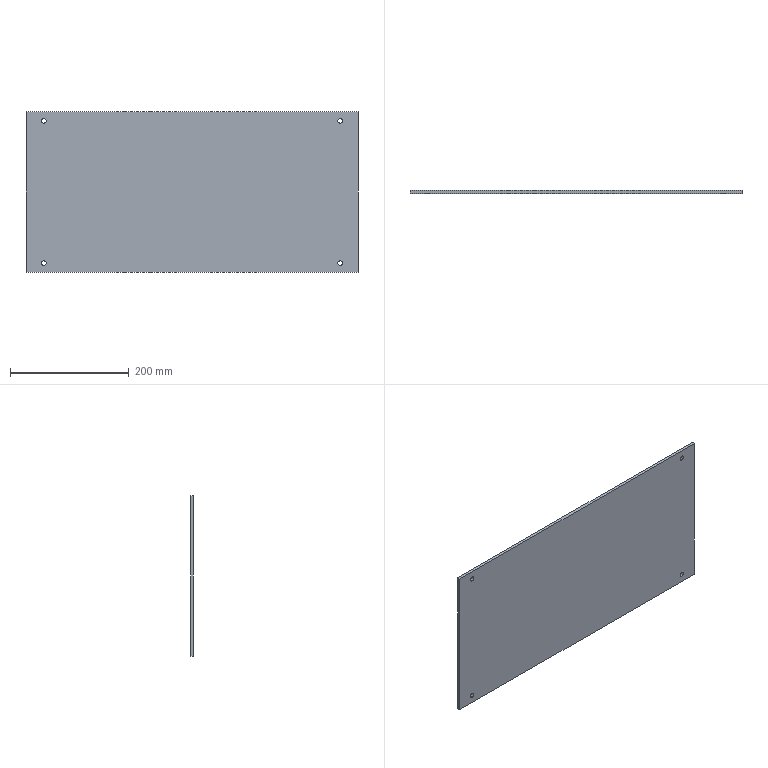Part | STEP file | OP10-004_front cover (L) | 1 solid | 14 faces | box 560 x 5 x 270 mm | volume 754995 mm3 | cylinder 8 | plane 6 | commonest cylinder face diameters 8 x8
STEP:
#1=CARTESIAN_POINT('',(0.,0.,0.));
#2=DIRECTION('',(0.,0.,1.));
#3=DIRECTION('',(1.,0.,0.));
#4=AXIS2_PLACEMENT_3D('',#1,#2,#3);
#5=CARTESIAN_POINT('',(250.,0.,124.));
#6=VERTEX_POINT('',#5);
#7=CARTESIAN_POINT('',(250.,5.,124.));
#8=VERTEX_POINT('',#7);
#9=CARTESIAN_POINT('',(250.,5.,124.));
#10=DIRECTION('',(0.,1.,0.));
#11=VECTOR('',#10,1.);
#12=LINE('',#9,#11);
#13=CARTESIAN_POINT('',(250.,5.,120.));
#14=DIRECTION('',(0.,1.,0.));
#15=DIRECTION('',(0.,0.,1.));
#16=AXIS2_PLACEMENT_3D('',#13,#14,#15);
#17=CYLINDRICAL_SURFACE('',#16,4.);
#18=CARTESIAN_POINT('',(6.283,0.));
#19=DIRECTION('',(0.,1.));
#20=VECTOR('',#19,1.);
#21=LINE('',#18,#20);
#22=(GEOMETRIC_REPRESENTATION_CONTEXT(2)PARAMETRIC_REPRESENTATION_CONTEXT()REPRESENTATION_CONTEXT('',''));
#23=DEFINITIONAL_REPRESENTATION('',(#21),#22);
#24=PCURVE('',#17,#23);
#25=CARTESIAN_POINT('',(250.,5.,120.));
#26=DIRECTION('',(0.,1.,0.));
#27=DIRECTION('',(0.,0.,1.));
#28=AXIS2_PLACEMENT_3D('',#25,#26,#27);
#29=CYLINDRICAL_SURFACE('',#28,4.);
#30=CARTESIAN_POINT('',(0.,0.));
#31=DIRECTION('',(0.,1.));
#32=VECTOR('',#31,1.);
#33=LINE('',#30,#32);
#34=(GEOMETRIC_REPRESENTATION_CONTEXT(2)PARAMETRIC_REPRESENTATION_CONTEXT()REPRESENTATION_CONTEXT('',''));
#35=DEFINITIONAL_REPRESENTATION('',(#33),#34);
#36=PCURVE('',#29,#35);
#37=SURFACE_CURVE('',#12,(#24,#36),.PCURVE_S1.);
#38=EDGE_CURVE('',#6,#8,#37,.T.);
#39=ORIENTED_EDGE('',*,*,#38,.T.);
#40=CARTESIAN_POINT('',(250.,5.,116.));
#41=VERTEX_POINT('',#40);
#42=CARTESIAN_POINT('',(250.,5.,120.));
#43=DIRECTION('',(0.,1.,0.));
#44=DIRECTION('',(0.,0.,1.));
#45=AXIS2_PLACEMENT_3D('',#42,#43,#44);
#46=CIRCLE('',#45,4.);
#47=CARTESIAN_POINT('',(0.,0.));
#48=DIRECTION('',(1.,0.));
#49=VECTOR('',#48,1.);
#50=LINE('',#47,#49);
#51=(GEOMETRIC_REPRESENTATION_CONTEXT(2)PARAMETRIC_REPRESENTATION_CONTEXT()REPRESENTATION_CONTEXT('',''));
#52=DEFINITIONAL_REPRESENTATION('',(#50),#51);
#53=PCURVE('',#17,#52);
#54=CARTESIAN_POINT('',(0.,5.,0.));
#55=DIRECTION('',(0.,-1.,0.));
#56=DIRECTION('',(0.,0.,-1.));
#57=AXIS2_PLACEMENT_3D('',#54,#55,#56);
#58=PLANE('',#57);
#59=CARTESIAN_POINT('',(-124.,250.));
#60=CARTESIAN_POINT('',(-124.,256.928));
#61=CARTESIAN_POINT('',(-118.,253.464));
#62=CARTESIAN_POINT('',(-112.,250.));
#63=CARTESIAN_POINT('',(-118.,246.536));
#64=CARTESIAN_POINT('',(-124.,243.072));
#65=CARTESIAN_POINT('',(-124.,250.));
#66=(BOUNDED_CURVE()B_SPLINE_CURVE(2,(#59,#60,#61,#62,#63,#64,#65),.UNSPECIFIED.,.T.,.F.)B_SPLINE_CURVE_WITH_KNOTS((1,2,2,2,2,1),(-2.094,0.,2.094,4.189,6.283,8.378),.UNSPECIFIED.)CURVE()GEOMETRIC_REPRESENTATION_ITEM()RATIONAL_B_SPLINE_CURVE((1.,0.5,1.,0.5,1.,0.5,1.))REPRESENTATION_ITEM(''));
#67=(GEOMETRIC_REPRESENTATION_CONTEXT(2)PARAMETRIC_REPRESENTATION_CONTEXT()REPRESENTATION_CONTEXT('',''));
#68=DEFINITIONAL_REPRESENTATION('',(#66),#67);
#69=PCURVE('',#58,#68);
#70=SURFACE_CURVE('',#46,(#53,#69),.PCURVE_S1.);
#71=EDGE_CURVE('',#41,#8,#70,.T.);
#72=ORIENTED_EDGE('',*,*,#71,.F.);
#73=CARTESIAN_POINT('',(250.,0.,116.));
#74=VERTEX_POINT('',#73);
#75=CARTESIAN_POINT('',(250.,5.,116.));
#76=DIRECTION('',(0.,1.,0.));
#77=VECTOR('',#76,1.);
#78=LINE('',#75,#77);
#79=CARTESIAN_POINT('',(3.142,0.));
#80=DIRECTION('',(0.,1.));
#81=VECTOR('',#80,1.);
#82=LINE('',#79,#81);
#83=(GEOMETRIC_REPRESENTATION_CONTEXT(2)PARAMETRIC_REPRESENTATION_CONTEXT()REPRESENTATION_CONTEXT('',''));
#84=DEFINITIONAL_REPRESENTATION('',(#82),#83);
#85=PCURVE('',#17,#84);
#86=CARTESIAN_POINT('',(3.142,0.));
#87=DIRECTION('',(0.,1.));
#88=VECTOR('',#87,1.);
#89=LINE('',#86,#88);
#90=(GEOMETRIC_REPRESENTATION_CONTEXT(2)PARAMETRIC_REPRESENTATION_CONTEXT()REPRESENTATION_CONTEXT('',''));
#91=DEFINITIONAL_REPRESENTATION('',(#89),#90);
#92=PCURVE('',#29,#91);
#93=SURFACE_CURVE('',#78,(#85,#92),.PCURVE_S1.);
#94=EDGE_CURVE('',#74,#41,#93,.T.);
#95=ORIENTED_EDGE('',*,*,#94,.F.);
#96=CARTESIAN_POINT('',(250.,0.,120.));
#97=DIRECTION('',(0.,-1.,0.));
#98=DIRECTION('',(0.,0.,-1.));
#99=AXIS2_PLACEMENT_3D('',#96,#97,#98);
#100=CIRCLE('',#99,4.);
#101=CARTESIAN_POINT('',(9.425,-5.));
#102=DIRECTION('',(-1.,0.));
#103=VECTOR('',#102,1.);
#104=LINE('',#101,#103);
#105=(GEOMETRIC_REPRESENTATION_CONTEXT(2)PARAMETRIC_REPRESENTATION_CONTEXT()REPRESENTATION_CONTEXT('',''));
#106=DEFINITIONAL_REPRESENTATION('',(#104),#105);
#107=PCURVE('',#17,#106);
#108=CARTESIAN_POINT('',(0.,0.,0.));
#109=DIRECTION('',(0.,-1.,0.));
#110=DIRECTION('',(0.,0.,-1.));
#111=AXIS2_PLACEMENT_3D('',#108,#109,#110);
#112=PLANE('',#111);
#113=CARTESIAN_POINT('',(-120.,250.));
#114=DIRECTION('',(1.,0.));
#115=AXIS2_PLACEMENT_2D('',#113,#114);
#116=CIRCLE('',#115,4.);
#117=(GEOMETRIC_REPRESENTATION_CONTEXT(2)PARAMETRIC_REPRESENTATION_CONTEXT()REPRESENTATION_CONTEXT('',''));
#118=DEFINITIONAL_REPRESENTATION('',(#116),#117);
#119=PCURVE('',#112,#118);
#120=SURFACE_CURVE('',#100,(#107,#119),.PCURVE_S1.);
#121=EDGE_CURVE('',#6,#74,#120,.T.);
#122=ORIENTED_EDGE('',*,*,#121,.F.);
#123=EDGE_LOOP('',(#39,#72,#95,#122));
#124=FACE_BOUND('',#123,.F.);
#125=ADVANCED_FACE('',(#124),#17,.F.);
#126=CARTESIAN_POINT('',(-250.,0.,124.));
#127=VERTEX_POINT('',#126);
#128=CARTESIAN_POINT('',(-250.,5.,124.));
#129=VERTEX_POINT('',#128);
#130=CARTESIAN_POINT('',(-250.,5.,124.));
#131=DIRECTION('',(0.,1.,0.));
#132=VECTOR('',#131,1.);
#133=LINE('',#130,#132);
#134=CARTESIAN_POINT('',(-250.,5.,120.));
#135=DIRECTION('',(0.,1.,0.));
#136=DIRECTION('',(0.,0.,1.));
#137=AXIS2_PLACEMENT_3D('',#134,#135,#136);
#138=CYLINDRICAL_SURFACE('',#137,4.);
#139=CARTESIAN_POINT('',(6.283,0.));
#140=DIRECTION('',(0.,1.));
#141=VECTOR('',#140,1.);
#142=LINE('',#139,#141);
#143=(GEOMETRIC_REPRESENTATION_CONTEXT(2)PARAMETRIC_REPRESENTATION_CONTEXT()REPRESENTATION_CONTEXT('',''));
#144=DEFINITIONAL_REPRESENTATION('',(#142),#143);
#145=PCURVE('',#138,#144);
#146=CARTESIAN_POINT('',(-250.,5.,120.));
#147=DIRECTION('',(0.,1.,0.));
#148=DIRECTION('',(0.,0.,1.));
#149=AXIS2_PLACEMENT_3D('',#146,#147,#148);
#150=CYLINDRICAL_SURFACE('',#149,4.);
#151=CARTESIAN_POINT('',(0.,0.));
#152=DIRECTION('',(0.,1.));
#153=VECTOR('',#152,1.);
#154=LINE('',#151,#153);
#155=(GEOMETRIC_REPRESENTATION_CONTEXT(2)PARAMETRIC_REPRESENTATION_CONTEXT()REPRESENTATION_CONTEXT('',''));
#156=DEFINITIONAL_REPRESENTATION('',(#154),#155);
#157=PCURVE('',#150,#156);
#158=SURFACE_CURVE('',#133,(#145,#157),.PCURVE_S1.);
#159=EDGE_CURVE('',#127,#129,#158,.T.);
#160=ORIENTED_EDGE('',*,*,#159,.T.);
#161=CARTESIAN_POINT('',(-250.,5.,116.));
#162=VERTEX_POINT('',#161);
#163=CARTESIAN_POINT('',(-250.,5.,120.));
#164=DIRECTION('',(0.,1.,0.));
#165=DIRECTION('',(0.,0.,1.));
#166=AXIS2_PLACEMENT_3D('',#163,#164,#165);
#167=CIRCLE('',#166,4.);
#168=CARTESIAN_POINT('',(0.,0.));
#169=DIRECTION('',(1.,0.));
#170=VECTOR('',#169,1.);
#171=LINE('',#168,#170);
#172=(GEOMETRIC_REPRESENTATION_CONTEXT(2)PARAMETRIC_REPRESENTATION_CONTEXT()REPRESENTATION_CONTEXT('',''));
#173=DEFINITIONAL_REPRESENTATION('',(#171),#172);
#174=PCURVE('',#138,#173);
#175=CARTESIAN_POINT('',(-124.,-250.));
#176=CARTESIAN_POINT('',(-124.,-243.072));
#177=CARTESIAN_POINT('',(-118.,-246.536));
#178=CARTESIAN_POINT('',(-112.,-250.));
#179=CARTESIAN_POINT('',(-118.,-253.464));
#180=CARTESIAN_POINT('',(-124.,-256.928));
#181=CARTESIAN_POINT('',(-124.,-250.));
#182=(BOUNDED_CURVE()B_SPLINE_CURVE(2,(#175,#176,#177,#178,#179,#180,#181),.UNSPECIFIED.,.T.,.F.)B_SPLINE_CURVE_WITH_KNOTS((1,2,2,2,2,1),(-2.094,0.,2.094,4.189,6.283,8.378),.UNSPECIFIED.)CURVE()GEOMETRIC_REPRESENTATION_ITEM()RATIONAL_B_SPLINE_CURVE((1.,0.5,1.,0.5,1.,0.5,1.))REPRESENTATION_ITEM(''));
#183=(GEOMETRIC_REPRESENTATION_CONTEXT(2)PARAMETRIC_REPRESENTATION_CONTEXT()REPRESENTATION_CONTEXT('',''));
#184=DEFINITIONAL_REPRESENTATION('',(#182),#183);
#185=PCURVE('',#58,#184);
#186=SURFACE_CURVE('',#167,(#174,#185),.PCURVE_S1.);
#187=EDGE_CURVE('',#162,#129,#186,.T.);
#188=ORIENTED_EDGE('',*,*,#187,.F.);
#189=CARTESIAN_POINT('',(-250.,0.,116.));
#190=VERTEX_POINT('',#189);
#191=CARTESIAN_POINT('',(-250.,5.,116.));
#192=DIRECTION('',(0.,1.,0.));
#193=VECTOR('',#192,1.);
#194=LINE('',#191,#193);
#195=CARTESIAN_POINT('',(3.142,0.));
#196=DIRECTION('',(0.,1.));
#197=VECTOR('',#196,1.);
#198=LINE('',#195,#197);
#199=(GEOMETRIC_REPRESENTATION_CONTEXT(2)PARAMETRIC_REPRESENTATION_CONTEXT()REPRESENTATION_CONTEXT('',''));
#200=DEFINITIONAL_REPRESENTATION('',(#198),#199);
#201=PCURVE('',#138,#200);
#202=CARTESIAN_POINT('',(3.142,0.));
#203=DIRECTION('',(0.,1.));
#204=VECTOR('',#203,1.);
#205=LINE('',#202,#204);
#206=(GEOMETRIC_REPRESENTATION_CONTEXT(2)PARAMETRIC_REPRESENTATION_CONTEXT()REPRESENTATION_CONTEXT('',''));
#207=DEFINITIONAL_REPRESENTATION('',(#205),#206);
#208=PCURVE('',#150,#207);
#209=SURFACE_CURVE('',#194,(#201,#208),.PCURVE_S1.);
#210=EDGE_CURVE('',#190,#162,#209,.T.);
#211=ORIENTED_EDGE('',*,*,#210,.F.);
#212=CARTESIAN_POINT('',(-250.,0.,120.));
#213=DIRECTION('',(0.,-1.,0.));
#214=DIRECTION('',(0.,0.,-1.));
#215=AXIS2_PLACEMENT_3D('',#212,#213,#214);
#216=CIRCLE('',#215,4.);
#217=CARTESIAN_POINT('',(9.425,-5.));
#218=DIRECTION('',(-1.,0.));
#219=VECTOR('',#218,1.);
#220=LINE('',#217,#219);
#221=(GEOMETRIC_REPRESENTATION_CONTEXT(2)PARAMETRIC_REPRESENTATION_CONTEXT()REPRESENTATION_CONTEXT('',''));
#222=DEFINITIONAL_REPRESENTATION('',(#220),#221);
#223=PCURVE('',#138,#222);
#224=CARTESIAN_POINT('',(-120.,-250.));
#225=DIRECTION('',(1.,0.));
#226=AXIS2_PLACEMENT_2D('',#224,#225);
#227=CIRCLE('',#226,4.);
#228=(GEOMETRIC_REPRESENTATION_CONTEXT(2)PARAMETRIC_REPRESENTATION_CONTEXT()REPRESENTATION_CONTEXT('',''));
#229=DEFINITIONAL_REPRESENTATION('',(#227),#228);
#230=PCURVE('',#112,#229);
#231=SURFACE_CURVE('',#216,(#223,#230),.PCURVE_S1.);
#232=EDGE_CURVE('',#127,#190,#231,.T.);
#233=ORIENTED_EDGE('',*,*,#232,.F.);
#234=EDGE_LOOP('',(#160,#188,#211,#233));
#235=FACE_BOUND('',#234,.F.);
#236=ADVANCED_FACE('',(#235),#138,.F.);
#237=CARTESIAN_POINT('',(250.,0.,-116.));
#238=VERTEX_POINT('',#237);
#239=CARTESIAN_POINT('',(250.,5.,-116.));
#240=VERTEX_POINT('',#239);
#241=CARTESIAN_POINT('',(250.,5.,-116.));
#242=DIRECTION('',(0.,1.,0.));
#243=VECTOR('',#242,1.);
#244=LINE('',#241,#243);
#245=CARTESIAN_POINT('',(250.,5.,-120.));
#246=DIRECTION('',(0.,1.,0.));
#247=DIRECTION('',(0.,0.,1.));
#248=AXIS2_PLACEMENT_3D('',#245,#246,#247);
#249=CYLINDRICAL_SURFACE('',#248,4.);
#250=CARTESIAN_POINT('',(6.283,0.));
#251=DIRECTION('',(0.,1.));
#252=VECTOR('',#251,1.);
#253=LINE('',#250,#252);
#254=(GEOMETRIC_REPRESENTATION_CONTEXT(2)PARAMETRIC_REPRESENTATION_CONTEXT()REPRESENTATION_CONTEXT('',''));
#255=DEFINITIONAL_REPRESENTATION('',(#253),#254);
#256=PCURVE('',#249,#255);
#257=CARTESIAN_POINT('',(250.,5.,-120.));
#258=DIRECTION('',(0.,1.,0.));
#259=DIRECTION('',(0.,0.,1.));
#260=AXIS2_PLACEMENT_3D('',#257,#258,#259);
#261=CYLINDRICAL_SURFACE('',#260,4.);
#262=CARTESIAN_POINT('',(0.,0.));
#263=DIRECTION('',(0.,1.));
#264=VECTOR('',#263,1.);
#265=LINE('',#262,#264);
#266=(GEOMETRIC_REPRESENTATION_CONTEXT(2)PARAMETRIC_REPRESENTATION_CONTEXT()REPRESENTATION_CONTEXT('',''));
#267=DEFINITIONAL_REPRESENTATION('',(#265),#266);
#268=PCURVE('',#261,#267);
#269=SURFACE_CURVE('',#244,(#256,#268),.PCURVE_S1.);
#270=EDGE_CURVE('',#238,#240,#269,.T.);
#271=ORIENTED_EDGE('',*,*,#270,.T.);
#272=CARTESIAN_POINT('',(250.,5.,-124.));
#273=VERTEX_POINT('',#272);
#274=CARTESIAN_POINT('',(250.,5.,-120.));
#275=DIRECTION('',(0.,1.,0.));
#276=DIRECTION('',(0.,0.,1.));
#277=AXIS2_PLACEMENT_3D('',#274,#275,#276);
#278=CIRCLE('',#277,4.);
#279=CARTESIAN_POINT('',(0.,0.));
#280=DIRECTION('',(1.,0.));
#281=VECTOR('',#280,1.);
#282=LINE('',#279,#281);
#283=(GEOMETRIC_REPRESENTATION_CONTEXT(2)PARAMETRIC_REPRESENTATION_CONTEXT()REPRESENTATION_CONTEXT('',''));
#284=DEFINITIONAL_REPRESENTATION('',(#282),#283);
#285=PCURVE('',#249,#284);
#286=CARTESIAN_POINT('',(116.,250.));
#287=CARTESIAN_POINT('',(116.,256.928));
#288=CARTESIAN_POINT('',(122.,253.464));
#289=CARTESIAN_POINT('',(128.,250.));
#290=CARTESIAN_POINT('',(122.,246.536));
#291=CARTESIAN_POINT('',(116.,243.072));
#292=CARTESIAN_POINT('',(116.,250.));
#293=(BOUNDED_CURVE()B_SPLINE_CURVE(2,(#286,#287,#288,#289,#290,#291,#292),.UNSPECIFIED.,.T.,.F.)B_SPLINE_CURVE_WITH_KNOTS((1,2,2,2,2,1),(-2.094,0.,2.094,4.189,6.283,8.378),.UNSPECIFIED.)CURVE()GEOMETRIC_REPRESENTATION_ITEM()RATIONAL_B_SPLINE_CURVE((1.,0.5,1.,0.5,1.,0.5,1.))REPRESENTATION_ITEM(''));
#294=(GEOMETRIC_REPRESENTATION_CONTEXT(2)PARAMETRIC_REPRESENTATION_CONTEXT()REPRESENTATION_CONTEXT('',''));
#295=DEFINITIONAL_REPRESENTATION('',(#293),#294);
#296=PCURVE('',#58,#295);
#297=SURFACE_CURVE('',#278,(#285,#296),.PCURVE_S1.);
#298=EDGE_CURVE('',#273,#240,#297,.T.);
#299=ORIENTED_EDGE('',*,*,#298,.F.);
#300=CARTESIAN_POINT('',(250.,0.,-124.));
#301=VERTEX_POINT('',#300);
#302=CARTESIAN_POINT('',(250.,5.,-124.));
#303=DIRECTION('',(0.,1.,0.));
#304=VECTOR('',#303,1.);
#305=LINE('',#302,#304);
#306=CARTESIAN_POINT('',(3.142,0.));
#307=DIRECTION('',(0.,1.));
#308=VECTOR('',#307,1.);
#309=LINE('',#306,#308);
#310=(GEOMETRIC_REPRESENTATION_CONTEXT(2)PARAMETRIC_REPRESENTATION_CONTEXT()REPRESENTATION_CONTEXT('',''));
#311=DEFINITIONAL_REPRESENTATION('',(#309),#310);
#312=PCURVE('',#249,#311);
#313=CARTESIAN_POINT('',(3.142,0.));
#314=DIRECTION('',(0.,1.));
#315=VECTOR('',#314,1.);
#316=LINE('',#313,#315);
#317=(GEOMETRIC_REPRESENTATION_CONTEXT(2)PARAMETRIC_REPRESENTATION_CONTEXT()REPRESENTATION_CONTEXT('',''));
#318=DEFINITIONAL_REPRESENTATION('',(#316),#317);
#319=PCURVE('',#261,#318);
#320=SURFACE_CURVE('',#305,(#312,#319),.PCURVE_S1.);
#321=EDGE_CURVE('',#301,#273,#320,.T.);
#322=ORIENTED_EDGE('',*,*,#321,.F.);
#323=CARTESIAN_POINT('',(250.,0.,-120.));
#324=DIRECTION('',(0.,-1.,0.));
#325=DIRECTION('',(0.,0.,-1.));
#326=AXIS2_PLACEMENT_3D('',#323,#324,#325);
#327=CIRCLE('',#326,4.);
#328=CARTESIAN_POINT('',(9.425,-5.));
#329=DIRECTION('',(-1.,0.));
#330=VECTOR('',#329,1.);
#331=LINE('',#328,#330);
#332=(GEOMETRIC_REPRESENTATION_CONTEXT(2)PARAMETRIC_REPRESENTATION_CONTEXT()REPRESENTATION_CONTEXT('',''));
#333=DEFINITIONAL_REPRESENTATION('',(#331),#332);
#334=PCURVE('',#249,#333);
#335=CARTESIAN_POINT('',(120.,250.));
#336=DIRECTION('',(1.,0.));
#337=AXIS2_PLACEMENT_2D('',#335,#336);
#338=CIRCLE('',#337,4.);
#339=(GEOMETRIC_REPRESENTATION_CONTEXT(2)PARAMETRIC_REPRESENTATION_CONTEXT()REPRESENTATION_CONTEXT('',''));
#340=DEFINITIONAL_REPRESENTATION('',(#338),#339);
#341=PCURVE('',#112,#340);
#342=SURFACE_CURVE('',#327,(#334,#341),.PCURVE_S1.);
#343=EDGE_CURVE('',#238,#301,#342,.T.);
#344=ORIENTED_EDGE('',*,*,#343,.F.);
#345=EDGE_LOOP('',(#271,#299,#322,#344));
#346=FACE_BOUND('',#345,.F.);
#347=ADVANCED_FACE('',(#346),#249,.F.);
#348=CARTESIAN_POINT('',(-250.,0.,-116.));
#349=VERTEX_POINT('',#348);
#350=CARTESIAN_POINT('',(-250.,5.,-116.));
#351=VERTEX_POINT('',#350);
#352=CARTESIAN_POINT('',(-250.,5.,-116.));
#353=DIRECTION('',(0.,1.,0.));
#354=VECTOR('',#353,1.);
#355=LINE('',#352,#354);
#356=CARTESIAN_POINT('',(-250.,5.,-120.));
#357=DIRECTION('',(0.,1.,0.));
#358=DIRECTION('',(0.,0.,1.));
#359=AXIS2_PLACEMENT_3D('',#356,#357,#358);
#360=CYLINDRICAL_SURFACE('',#359,4.);
#361=CARTESIAN_POINT('',(6.283,0.));
#362=DIRECTION('',(0.,1.));
#363=VECTOR('',#362,1.);
#364=LINE('',#361,#363);
#365=(GEOMETRIC_REPRESENTATION_CONTEXT(2)PARAMETRIC_REPRESENTATION_CONTEXT()REPRESENTATION_CONTEXT('',''));
#366=DEFINITIONAL_REPRESENTATION('',(#364),#365);
#367=PCURVE('',#360,#366);
#368=CARTESIAN_POINT('',(-250.,5.,-120.));
#369=DIRECTION('',(0.,1.,0.));
#370=DIRECTION('',(0.,0.,1.));
#371=AXIS2_PLACEMENT_3D('',#368,#369,#370);
#372=CYLINDRICAL_SURFACE('',#371,4.);
#373=CARTESIAN_POINT('',(0.,0.));
#374=DIRECTION('',(0.,1.));
#375=VECTOR('',#374,1.);
#376=LINE('',#373,#375);
#377=(GEOMETRIC_REPRESENTATION_CONTEXT(2)PARAMETRIC_REPRESENTATION_CONTEXT()REPRESENTATION_CONTEXT('',''));
#378=DEFINITIONAL_REPRESENTATION('',(#376),#377);
#379=PCURVE('',#372,#378);
#380=SURFACE_CURVE('',#355,(#367,#379),.PCURVE_S1.);
#381=EDGE_CURVE('',#349,#351,#380,.T.);
#382=ORIENTED_EDGE('',*,*,#381,.T.);
#383=CARTESIAN_POINT('',(-250.,5.,-124.));
#384=VERTEX_POINT('',#383);
#385=CARTESIAN_POINT('',(-250.,5.,-120.));
#386=DIRECTION('',(0.,1.,0.));
#387=DIRECTION('',(0.,0.,1.));
#388=AXIS2_PLACEMENT_3D('',#385,#386,#387);
#389=CIRCLE('',#388,4.);
#390=CARTESIAN_POINT('',(0.,0.));
#391=DIRECTION('',(1.,0.));
#392=VECTOR('',#391,1.);
#393=LINE('',#390,#392);
#394=(GEOMETRIC_REPRESENTATION_CONTEXT(2)PARAMETRIC_REPRESENTATION_CONTEXT()REPRESENTATION_CONTEXT('',''));
#395=DEFINITIONAL_REPRESENTATION('',(#393),#394);
#396=PCURVE('',#360,#395);
#397=CARTESIAN_POINT('',(116.,-250.));
#398=CARTESIAN_POINT('',(116.,-243.072));
#399=CARTESIAN_POINT('',(122.,-246.536));
#400=CARTESIAN_POINT('',(128.,-250.));
#401=CARTESIAN_POINT('',(122.,-253.464));
#402=CARTESIAN_POINT('',(116.,-256.928));
#403=CARTESIAN_POINT('',(116.,-250.));
#404=(BOUNDED_CURVE()B_SPLINE_CURVE(2,(#397,#398,#399,#400,#401,#402,#403),.UNSPECIFIED.,.T.,.F.)B_SPLINE_CURVE_WITH_KNOTS((1,2,2,2,2,1),(-2.094,0.,2.094,4.189,6.283,8.378),.UNSPECIFIED.)CURVE()GEOMETRIC_REPRESENTATION_ITEM()RATIONAL_B_SPLINE_CURVE((1.,0.5,1.,0.5,1.,0.5,1.))REPRESENTATION_ITEM(''));
#405=(GEOMETRIC_REPRESENTATION_CONTEXT(2)PARAMETRIC_REPRESENTATION_CONTEXT()REPRESENTATION_CONTEXT('',''));
#406=DEFINITIONAL_REPRESENTATION('',(#404),#405);
#407=PCURVE('',#58,#406);
#408=SURFACE_CURVE('',#389,(#396,#407),.PCURVE_S1.);
#409=EDGE_CURVE('',#384,#351,#408,.T.);
#410=ORIENTED_EDGE('',*,*,#409,.F.);
#411=CARTESIAN_POINT('',(-250.,0.,-124.));
#412=VERTEX_POINT('',#411);
#413=CARTESIAN_POINT('',(-250.,5.,-124.));
#414=DIRECTION('',(0.,1.,0.));
#415=VECTOR('',#414,1.);
#416=LINE('',#413,#415);
#417=CARTESIAN_POINT('',(3.142,0.));
#418=DIRECTION('',(0.,1.));
#419=VECTOR('',#418,1.);
#420=LINE('',#417,#419);
#421=(GEOMETRIC_REPRESENTATION_CONTEXT(2)PARAMETRIC_REPRESENTATION_CONTEXT()REPRESENTATION_CONTEXT('',''));
#422=DEFINITIONAL_REPRESENTATION('',(#420),#421);
#423=PCURVE('',#360,#422);
#424=CARTESIAN_POINT('',(3.142,0.));
#425=DIRECTION('',(0.,1.));
#426=VECTOR('',#425,1.);
#427=LINE('',#424,#426);
#428=(GEOMETRIC_REPRESENTATION_CONTEXT(2)PARAMETRIC_REPRESENTATION_CONTEXT()REPRESENTATION_CONTEXT('',''));
#429=DEFINITIONAL_REPRESENTATION('',(#427),#428);
#430=PCURVE('',#372,#429);
#431=SURFACE_CURVE('',#416,(#423,#430),.PCURVE_S1.);
#432=EDGE_CURVE('',#412,#384,#431,.T.);
#433=ORIENTED_EDGE('',*,*,#432,.F.);
#434=CARTESIAN_POINT('',(-250.,0.,-120.));
#435=DIRECTION('',(0.,-1.,0.));
#436=DIRECTION('',(0.,0.,-1.));
#437=AXIS2_PLACEMENT_3D('',#434,#435,#436);
#438=CIRCLE('',#437,4.);
#439=CARTESIAN_POINT('',(9.425,-5.));
#440=DIRECTION('',(-1.,0.));
#441=VECTOR('',#440,1.);
#442=LINE('',#439,#441);
#443=(GEOMETRIC_REPRESENTATION_CONTEXT(2)PARAMETRIC_REPRESENTATION_CONTEXT()REPRESENTATION_CONTEXT('',''));
#444=DEFINITIONAL_REPRESENTATION('',(#442),#443);
#445=PCURVE('',#360,#444);
#446=CARTESIAN_POINT('',(120.,-250.));
#447=DIRECTION('',(1.,0.));
#448=AXIS2_PLACEMENT_2D('',#446,#447);
#449=CIRCLE('',#448,4.);
#450=(GEOMETRIC_REPRESENTATION_CONTEXT(2)PARAMETRIC_REPRESENTATION_CONTEXT()REPRESENTATION_CONTEXT('',''));
#451=DEFINITIONAL_REPRESENTATION('',(#449),#450);
#452=PCURVE('',#112,#451);
#453=SURFACE_CURVE('',#438,(#445,#452),.PCURVE_S1.);
#454=EDGE_CURVE('',#349,#412,#453,.T.);
#455=ORIENTED_EDGE('',*,*,#454,.F.);
#456=EDGE_LOOP('',(#382,#410,#433,#455));
#457=FACE_BOUND('',#456,.F.);
#458=ADVANCED_FACE('',(#457),#360,.F.);
#459=CARTESIAN_POINT('',(280.,0.,135.));
#460=VERTEX_POINT('',#459);
#461=CARTESIAN_POINT('',(280.,0.,-135.));
#462=VERTEX_POINT('',#461);
#463=CARTESIAN_POINT('',(280.,0.,135.));
#464=DIRECTION('',(0.,0.,-1.));
#465=VECTOR('',#464,1.);
#466=LINE('',#463,#465);
#467=CARTESIAN_POINT('',(280.,5.,135.));
#468=DIRECTION('',(-1.,0.,0.));
#469=DIRECTION('',(0.,0.,1.));
#470=AXIS2_PLACEMENT_3D('',#467,#468,#469);
#471=PLANE('',#470);
#472=CARTESIAN_POINT('',(0.,-5.));
#473=DIRECTION('',(-1.,0.));
#474=VECTOR('',#473,1.);
#475=LINE('',#472,#474);
#476=(GEOMETRIC_REPRESENTATION_CONTEXT(2)PARAMETRIC_REPRESENTATION_CONTEXT()REPRESENTATION_CONTEXT('',''));
#477=DEFINITIONAL_REPRESENTATION('',(#475),#476);
#478=PCURVE('',#471,#477);
#479=CARTESIAN_POINT('',(-135.,280.));
#480=DIRECTION('',(1.,0.));
#481=VECTOR('',#480,1.);
#482=LINE('',#479,#481);
#483=(GEOMETRIC_REPRESENTATION_CONTEXT(2)PARAMETRIC_REPRESENTATION_CONTEXT()REPRESENTATION_CONTEXT('',''));
#484=DEFINITIONAL_REPRESENTATION('',(#482),#483);
#485=PCURVE('',#112,#484);
#486=SURFACE_CURVE('',#466,(#478,#485),.PCURVE_S1.);
#487=EDGE_CURVE('',#460,#462,#486,.T.);
#488=ORIENTED_EDGE('',*,*,#487,.T.);
#489=CARTESIAN_POINT('',(280.,5.,-135.));
#490=VERTEX_POINT('',#489);
#491=CARTESIAN_POINT('',(280.,5.,-135.));
#492=DIRECTION('',(0.,-1.,0.));
#493=VECTOR('',#492,1.);
#494=LINE('',#491,#493);
#495=CARTESIAN_POINT('',(-270.,0.));
#496=DIRECTION('',(0.,-1.));
#497=VECTOR('',#496,1.);
#498=LINE('',#495,#497);
#499=(GEOMETRIC_REPRESENTATION_CONTEXT(2)PARAMETRIC_REPRESENTATION_CONTEXT()REPRESENTATION_CONTEXT('',''));
#500=DEFINITIONAL_REPRESENTATION('',(#498),#499);
#501=PCURVE('',#471,#500);
#502=CARTESIAN_POINT('',(-280.,5.,-135.));
#503=DIRECTION('',(0.,0.,1.));
#504=DIRECTION('',(1.,0.,0.));
#505=AXIS2_PLACEMENT_3D('',#502,#503,#504);
#506=PLANE('',#505);
#507=CARTESIAN_POINT('',(560.,0.));
#508=DIRECTION('',(0.,-1.));
#509=VECTOR('',#508,1.);
#510=LINE('',#507,#509);
#511=(GEOMETRIC_REPRESENTATION_CONTEXT(2)PARAMETRIC_REPRESENTATION_CONTEXT()REPRESENTATION_CONTEXT('',''));
#512=DEFINITIONAL_REPRESENTATION('',(#510),#511);
#513=PCURVE('',#506,#512);
#514=SURFACE_CURVE('',#494,(#501,#513),.PCURVE_S1.);
#515=EDGE_CURVE('',#490,#462,#514,.T.);
#516=ORIENTED_EDGE('',*,*,#515,.F.);
#517=CARTESIAN_POINT('',(280.,5.,135.));
#518=VERTEX_POINT('',#517);
#519=CARTESIAN_POINT('',(280.,5.,135.));
#520=DIRECTION('',(0.,0.,-1.));
#521=VECTOR('',#520,1.);
#522=LINE('',#519,#521);
#523=CARTESIAN_POINT('',(0.,0.));
#524=DIRECTION('',(-1.,0.));
#525=VECTOR('',#524,1.);
#526=LINE('',#523,#525);
#527=(GEOMETRIC_REPRESENTATION_CONTEXT(2)PARAMETRIC_REPRESENTATION_CONTEXT()REPRESENTATION_CONTEXT('',''));
#528=DEFINITIONAL_REPRESENTATION('',(#526),#527);
#529=PCURVE('',#471,#528);
#530=CARTESIAN_POINT('',(-135.,280.));
#531=DIRECTION('',(1.,0.));
#532=VECTOR('',#531,1.);
#533=LINE('',#530,#532);
#534=(GEOMETRIC_REPRESENTATION_CONTEXT(2)PARAMETRIC_REPRESENTATION_CONTEXT()REPRESENTATION_CONTEXT('',''));
#535=DEFINITIONAL_REPRESENTATION('',(#533),#534);
#536=PCURVE('',#58,#535);
#537=SURFACE_CURVE('',#522,(#529,#536),.PCURVE_S1.);
#538=EDGE_CURVE('',#518,#490,#537,.T.);
#539=ORIENTED_EDGE('',*,*,#538,.F.);
#540=CARTESIAN_POINT('',(280.,5.,135.));
#541=DIRECTION('',(0.,-1.,0.));
#542=VECTOR('',#541,1.);
#543=LINE('',#540,#542);
#544=CARTESIAN_POINT('',(0.,0.));
#545=DIRECTION('',(0.,-1.));
#546=VECTOR('',#545,1.);
#547=LINE('',#544,#546);
#548=(GEOMETRIC_REPRESENTATION_CONTEXT(2)PARAMETRIC_REPRESENTATION_CONTEXT()REPRESENTATION_CONTEXT('',''));
#549=DEFINITIONAL_REPRESENTATION('',(#547),#548);
#550=PCURVE('',#471,#549);
#551=CARTESIAN_POINT('',(-280.,5.,135.));
#552=DIRECTION('',(0.,0.,-1.));
#553=DIRECTION('',(-1.,0.,0.));
#554=AXIS2_PLACEMENT_3D('',#551,#552,#553);
#555=PLANE('',#554);
#556=CARTESIAN_POINT('',(-560.,0.));
#557=DIRECTION('',(0.,-1.));
#558=VECTOR('',#557,1.);
#559=LINE('',#556,#558);
#560=(GEOMETRIC_REPRESENTATION_CONTEXT(2)PARAMETRIC_REPRESENTATION_CONTEXT()REPRESENTATION_CONTEXT('',''));
#561=DEFINITIONAL_REPRESENTATION('',(#559),#560);
#562=PCURVE('',#555,#561);
#563=SURFACE_CURVE('',#543,(#550,#562),.PCURVE_S1.);
#564=EDGE_CURVE('',#518,#460,#563,.T.);
#565=ORIENTED_EDGE('',*,*,#564,.T.);
#566=EDGE_LOOP('',(#488,#516,#539,#565));
#567=FACE_BOUND('',#566,.T.);
#568=ADVANCED_FACE('',(#567),#471,.F.);
#569=CARTESIAN_POINT('',(-280.,0.,-135.));
#570=VERTEX_POINT('',#569);
#571=CARTESIAN_POINT('',(-280.,0.,-135.));
#572=DIRECTION('',(-1.,0.,0.));
#573=VECTOR('',#572,1.);
#574=LINE('',#571,#573);
#575=CARTESIAN_POINT('',(0.,-5.));
#576=DIRECTION('',(-1.,0.));
#577=VECTOR('',#576,1.);
#578=LINE('',#575,#577);
#579=(GEOMETRIC_REPRESENTATION_CONTEXT(2)PARAMETRIC_REPRESENTATION_CONTEXT()REPRESENTATION_CONTEXT('',''));
#580=DEFINITIONAL_REPRESENTATION('',(#578),#579);
#581=PCURVE('',#506,#580);
#582=CARTESIAN_POINT('',(135.,-280.));
#583=DIRECTION('',(0.,-1.));
#584=VECTOR('',#583,1.);
#585=LINE('',#582,#584);
#586=(GEOMETRIC_REPRESENTATION_CONTEXT(2)PARAMETRIC_REPRESENTATION_CONTEXT()REPRESENTATION_CONTEXT('',''));
#587=DEFINITIONAL_REPRESENTATION('',(#585),#586);
#588=PCURVE('',#112,#587);
#589=SURFACE_CURVE('',#574,(#581,#588),.PCURVE_S1.);
#590=EDGE_CURVE('',#462,#570,#589,.T.);
#591=ORIENTED_EDGE('',*,*,#590,.T.);
#592=CARTESIAN_POINT('',(-280.,5.,-135.));
#593=VERTEX_POINT('',#592);
#594=CARTESIAN_POINT('',(-280.,5.,-135.));
#595=DIRECTION('',(0.,-1.,0.));
#596=VECTOR('',#595,1.);
#597=LINE('',#594,#596);
#598=CARTESIAN_POINT('',(0.,0.));
#599=DIRECTION('',(0.,-1.));
#600=VECTOR('',#599,1.);
#601=LINE('',#598,#600);
#602=(GEOMETRIC_REPRESENTATION_CONTEXT(2)PARAMETRIC_REPRESENTATION_CONTEXT()REPRESENTATION_CONTEXT('',''));
#603=DEFINITIONAL_REPRESENTATION('',(#601),#602);
#604=PCURVE('',#506,#603);
#605=CARTESIAN_POINT('',(-280.,5.,135.));
#606=DIRECTION('',(1.,0.,0.));
#607=DIRECTION('',(0.,0.,-1.));
#608=AXIS2_PLACEMENT_3D('',#605,#606,#607);
#609=PLANE('',#608);
#610=CARTESIAN_POINT('',(270.,0.));
#611=DIRECTION('',(0.,-1.));
#612=VECTOR('',#611,1.);
#613=LINE('',#610,#612);
#614=(GEOMETRIC_REPRESENTATION_CONTEXT(2)PARAMETRIC_REPRESENTATION_CONTEXT()REPRESENTATION_CONTEXT('',''));
#615=DEFINITIONAL_REPRESENTATION('',(#613),#614);
#616=PCURVE('',#609,#615);
#617=SURFACE_CURVE('',#597,(#604,#616),.PCURVE_S1.);
#618=EDGE_CURVE('',#593,#570,#617,.T.);
#619=ORIENTED_EDGE('',*,*,#618,.F.);
#620=CARTESIAN_POINT('',(-280.,5.,-135.));
#621=DIRECTION('',(-1.,0.,0.));
#622=VECTOR('',#621,1.);
#623=LINE('',#620,#622);
#624=CARTESIAN_POINT('',(0.,0.));
#625=DIRECTION('',(-1.,0.));
#626=VECTOR('',#625,1.);
#627=LINE('',#624,#626);
#628=(GEOMETRIC_REPRESENTATION_CONTEXT(2)PARAMETRIC_REPRESENTATION_CONTEXT()REPRESENTATION_CONTEXT('',''));
#629=DEFINITIONAL_REPRESENTATION('',(#627),#628);
#630=PCURVE('',#506,#629);
#631=CARTESIAN_POINT('',(135.,-280.));
#632=DIRECTION('',(0.,-1.));
#633=VECTOR('',#632,1.);
#634=LINE('',#631,#633);
#635=(GEOMETRIC_REPRESENTATION_CONTEXT(2)PARAMETRIC_REPRESENTATION_CONTEXT()REPRESENTATION_CONTEXT('',''));
#636=DEFINITIONAL_REPRESENTATION('',(#634),#635);
#637=PCURVE('',#58,#636);
#638=SURFACE_CURVE('',#623,(#630,#637),.PCURVE_S1.);
#639=EDGE_CURVE('',#490,#593,#638,.T.);
#640=ORIENTED_EDGE('',*,*,#639,.F.);
#641=ORIENTED_EDGE('',*,*,#515,.T.);
#642=EDGE_LOOP('',(#591,#619,#640,#641));
#643=FACE_BOUND('',#642,.T.);
#644=ADVANCED_FACE('',(#643),#506,.F.);
#645=CARTESIAN_POINT('',(-280.,0.,135.));
#646=VERTEX_POINT('',#645);
#647=CARTESIAN_POINT('',(-280.,0.,135.));
#648=DIRECTION('',(0.,0.,1.));
#649=VECTOR('',#648,1.);
#650=LINE('',#647,#649);
#651=CARTESIAN_POINT('',(0.,-5.));
#652=DIRECTION('',(-1.,0.));
#653=VECTOR('',#652,1.);
#654=LINE('',#651,#653);
#655=(GEOMETRIC_REPRESENTATION_CONTEXT(2)PARAMETRIC_REPRESENTATION_CONTEXT()REPRESENTATION_CONTEXT('',''));
#656=DEFINITIONAL_REPRESENTATION('',(#654),#655);
#657=PCURVE('',#609,#656);
#658=CARTESIAN_POINT('',(-135.,-280.));
#659=DIRECTION('',(-1.,0.));
#660=VECTOR('',#659,1.);
#661=LINE('',#658,#660);
#662=(GEOMETRIC_REPRESENTATION_CONTEXT(2)PARAMETRIC_REPRESENTATION_CONTEXT()REPRESENTATION_CONTEXT('',''));
#663=DEFINITIONAL_REPRESENTATION('',(#661),#662);
#664=PCURVE('',#112,#663);
#665=SURFACE_CURVE('',#650,(#657,#664),.PCURVE_S1.);
#666=EDGE_CURVE('',#570,#646,#665,.T.);
#667=ORIENTED_EDGE('',*,*,#666,.T.);
#668=CARTESIAN_POINT('',(-280.,5.,135.));
#669=VERTEX_POINT('',#668);
#670=CARTESIAN_POINT('',(-280.,5.,135.));
#671=DIRECTION('',(0.,-1.,0.));
#672=VECTOR('',#671,1.);
#673=LINE('',#670,#672);
#674=CARTESIAN_POINT('',(0.,0.));
#675=DIRECTION('',(0.,-1.));
#676=VECTOR('',#675,1.);
#677=LINE('',#674,#676);
#678=(GEOMETRIC_REPRESENTATION_CONTEXT(2)PARAMETRIC_REPRESENTATION_CONTEXT()REPRESENTATION_CONTEXT('',''));
#679=DEFINITIONAL_REPRESENTATION('',(#677),#678);
#680=PCURVE('',#609,#679);
#681=CARTESIAN_POINT('',(0.,0.));
#682=DIRECTION('',(0.,-1.));
#683=VECTOR('',#682,1.);
#684=LINE('',#681,#683);
#685=(GEOMETRIC_REPRESENTATION_CONTEXT(2)PARAMETRIC_REPRESENTATION_CONTEXT()REPRESENTATION_CONTEXT('',''));
#686=DEFINITIONAL_REPRESENTATION('',(#684),#685);
#687=PCURVE('',#555,#686);
#688=SURFACE_CURVE('',#673,(#680,#687),.PCURVE_S1.);
#689=EDGE_CURVE('',#669,#646,#688,.T.);
#690=ORIENTED_EDGE('',*,*,#689,.F.);
#691=CARTESIAN_POINT('',(-280.,5.,135.));
#692=DIRECTION('',(0.,0.,1.));
#693=VECTOR('',#692,1.);
#694=LINE('',#691,#693);
#695=CARTESIAN_POINT('',(0.,0.));
#696=DIRECTION('',(-1.,0.));
#697=VECTOR('',#696,1.);
#698=LINE('',#695,#697);
#699=(GEOMETRIC_REPRESENTATION_CONTEXT(2)PARAMETRIC_REPRESENTATION_CONTEXT()REPRESENTATION_CONTEXT('',''));
#700=DEFINITIONAL_REPRESENTATION('',(#698),#699);
#701=PCURVE('',#609,#700);
#702=CARTESIAN_POINT('',(-135.,-280.));
#703=DIRECTION('',(-1.,0.));
#704=VECTOR('',#703,1.);
#705=LINE('',#702,#704);
#706=(GEOMETRIC_REPRESENTATION_CONTEXT(2)PARAMETRIC_REPRESENTATION_CONTEXT()REPRESENTATION_CONTEXT('',''));
#707=DEFINITIONAL_REPRESENTATION('',(#705),#706);
#708=PCURVE('',#58,#707);
#709=SURFACE_CURVE('',#694,(#701,#708),.PCURVE_S1.);
#710=EDGE_CURVE('',#593,#669,#709,.T.);
#711=ORIENTED_EDGE('',*,*,#710,.F.);
#712=ORIENTED_EDGE('',*,*,#618,.T.);
#713=EDGE_LOOP('',(#667,#690,#711,#712));
#714=FACE_BOUND('',#713,.T.);
#715=ADVANCED_FACE('',(#714),#609,.F.);
#716=CARTESIAN_POINT('',(-280.,0.,135.));
#717=DIRECTION('',(1.,0.,0.));
#718=VECTOR('',#717,1.);
#719=LINE('',#716,#718);
#720=CARTESIAN_POINT('',(0.,-5.));
#721=DIRECTION('',(-1.,0.));
#722=VECTOR('',#721,1.);
#723=LINE('',#720,#722);
#724=(GEOMETRIC_REPRESENTATION_CONTEXT(2)PARAMETRIC_REPRESENTATION_CONTEXT()REPRESENTATION_CONTEXT('',''));
#725=DEFINITIONAL_REPRESENTATION('',(#723),#724);
#726=PCURVE('',#555,#725);
#727=CARTESIAN_POINT('',(-135.,-280.));
#728=DIRECTION('',(0.,1.));
#729=VECTOR('',#728,1.);
#730=LINE('',#727,#729);
#731=(GEOMETRIC_REPRESENTATION_CONTEXT(2)PARAMETRIC_REPRESENTATION_CONTEXT()REPRESENTATION_CONTEXT('',''));
#732=DEFINITIONAL_REPRESENTATION('',(#730),#731);
#733=PCURVE('',#112,#732);
#734=SURFACE_CURVE('',#719,(#726,#733),.PCURVE_S1.);
#735=EDGE_CURVE('',#646,#460,#734,.T.);
#736=ORIENTED_EDGE('',*,*,#735,.T.);
#737=ORIENTED_EDGE('',*,*,#564,.F.);
#738=CARTESIAN_POINT('',(-280.,5.,135.));
#739=DIRECTION('',(1.,0.,0.));
#740=VECTOR('',#739,1.);
#741=LINE('',#738,#740);
#742=CARTESIAN_POINT('',(0.,0.));
#743=DIRECTION('',(-1.,0.));
#744=VECTOR('',#743,1.);
#745=LINE('',#742,#744);
#746=(GEOMETRIC_REPRESENTATION_CONTEXT(2)PARAMETRIC_REPRESENTATION_CONTEXT()REPRESENTATION_CONTEXT('',''));
#747=DEFINITIONAL_REPRESENTATION('',(#745),#746);
#748=PCURVE('',#555,#747);
#749=CARTESIAN_POINT('',(-135.,-280.));
#750=DIRECTION('',(0.,1.));
#751=VECTOR('',#750,1.);
#752=LINE('',#749,#751);
#753=(GEOMETRIC_REPRESENTATION_CONTEXT(2)PARAMETRIC_REPRESENTATION_CONTEXT()REPRESENTATION_CONTEXT('',''));
#754=DEFINITIONAL_REPRESENTATION('',(#752),#753);
#755=PCURVE('',#58,#754);
#756=SURFACE_CURVE('',#741,(#748,#755),.PCURVE_S1.);
#757=EDGE_CURVE('',#669,#518,#756,.T.);
#758=ORIENTED_EDGE('',*,*,#757,.F.);
#759=ORIENTED_EDGE('',*,*,#689,.T.);
#760=EDGE_LOOP('',(#736,#737,#758,#759));
#761=FACE_BOUND('',#760,.T.);
#762=ADVANCED_FACE('',(#761),#555,.F.);
#763=CARTESIAN_POINT('',(250.,5.,-120.));
#764=DIRECTION('',(0.,1.,0.));
#765=DIRECTION('',(0.,0.,1.));
#766=AXIS2_PLACEMENT_3D('',#763,#764,#765);
#767=CIRCLE('',#766,4.);
#768=CARTESIAN_POINT('',(116.,250.));
#769=CARTESIAN_POINT('',(116.,256.928));
#770=CARTESIAN_POINT('',(122.,253.464));
#771=CARTESIAN_POINT('',(128.,250.));
#772=CARTESIAN_POINT('',(122.,246.536));
#773=CARTESIAN_POINT('',(116.,243.072));
#774=CARTESIAN_POINT('',(116.,250.));
#775=(BOUNDED_CURVE()B_SPLINE_CURVE(2,(#768,#769,#770,#771,#772,#773,#774),.UNSPECIFIED.,.T.,.F.)B_SPLINE_CURVE_WITH_KNOTS((1,2,2,2,2,1),(-2.094,0.,2.094,4.189,6.283,8.378),.UNSPECIFIED.)CURVE()GEOMETRIC_REPRESENTATION_ITEM()RATIONAL_B_SPLINE_CURVE((1.,0.5,1.,0.5,1.,0.5,1.))REPRESENTATION_ITEM(''));
#776=(GEOMETRIC_REPRESENTATION_CONTEXT(2)PARAMETRIC_REPRESENTATION_CONTEXT()REPRESENTATION_CONTEXT('',''));
#777=DEFINITIONAL_REPRESENTATION('',(#775),#776);
#778=PCURVE('',#58,#777);
#779=CARTESIAN_POINT('',(0.,0.));
#780=DIRECTION('',(1.,0.));
#781=VECTOR('',#780,1.);
#782=LINE('',#779,#781);
#783=(GEOMETRIC_REPRESENTATION_CONTEXT(2)PARAMETRIC_REPRESENTATION_CONTEXT()REPRESENTATION_CONTEXT('',''));
#784=DEFINITIONAL_REPRESENTATION('',(#782),#783);
#785=PCURVE('',#261,#784);
#786=SURFACE_CURVE('',#767,(#778,#785),.PCURVE_S1.);
#787=EDGE_CURVE('',#240,#273,#786,.T.);
#788=ORIENTED_EDGE('',*,*,#787,.F.);
#789=ORIENTED_EDGE('',*,*,#298,.F.);
#790=EDGE_LOOP('',(#788,#789));
#791=FACE_BOUND('',#790,.T.);
#792=CARTESIAN_POINT('',(-250.,5.,-120.));
#793=DIRECTION('',(0.,1.,0.));
#794=DIRECTION('',(0.,0.,1.));
#795=AXIS2_PLACEMENT_3D('',#792,#793,#794);
#796=CIRCLE('',#795,4.);
#797=CARTESIAN_POINT('',(116.,-250.));
#798=CARTESIAN_POINT('',(116.,-243.072));
#799=CARTESIAN_POINT('',(122.,-246.536));
#800=CARTESIAN_POINT('',(128.,-250.));
#801=CARTESIAN_POINT('',(122.,-253.464));
#802=CARTESIAN_POINT('',(116.,-256.928));
#803=CARTESIAN_POINT('',(116.,-250.));
#804=(BOUNDED_CURVE()B_SPLINE_CURVE(2,(#797,#798,#799,#800,#801,#802,#803),.UNSPECIFIED.,.T.,.F.)B_SPLINE_CURVE_WITH_KNOTS((1,2,2,2,2,1),(-2.094,0.,2.094,4.189,6.283,8.378),.UNSPECIFIED.)CURVE()GEOMETRIC_REPRESENTATION_ITEM()RATIONAL_B_SPLINE_CURVE((1.,0.5,1.,0.5,1.,0.5,1.))REPRESENTATION_ITEM(''));
#805=(GEOMETRIC_REPRESENTATION_CONTEXT(2)PARAMETRIC_REPRESENTATION_CONTEXT()REPRESENTATION_CONTEXT('',''));
#806=DEFINITIONAL_REPRESENTATION('',(#804),#805);
#807=PCURVE('',#58,#806);
#808=CARTESIAN_POINT('',(0.,0.));
#809=DIRECTION('',(1.,0.));
#810=VECTOR('',#809,1.);
#811=LINE('',#808,#810);
#812=(GEOMETRIC_REPRESENTATION_CONTEXT(2)PARAMETRIC_REPRESENTATION_CONTEXT()REPRESENTATION_CONTEXT('',''));
#813=DEFINITIONAL_REPRESENTATION('',(#811),#812);
#814=PCURVE('',#372,#813);
#815=SURFACE_CURVE('',#796,(#807,#814),.PCURVE_S1.);
#816=EDGE_CURVE('',#351,#384,#815,.T.);
#817=ORIENTED_EDGE('',*,*,#816,.F.);
#818=ORIENTED_EDGE('',*,*,#409,.F.);
#819=EDGE_LOOP('',(#817,#818));
#820=FACE_BOUND('',#819,.T.);
#821=ORIENTED_EDGE('',*,*,#538,.T.);
#822=ORIENTED_EDGE('',*,*,#639,.T.);
#823=ORIENTED_EDGE('',*,*,#710,.T.);
#824=ORIENTED_EDGE('',*,*,#757,.T.);
#825=EDGE_LOOP('',(#821,#822,#823,#824));
#826=FACE_BOUND('',#825,.T.);
#827=CARTESIAN_POINT('',(-250.,5.,120.));
#828=DIRECTION('',(0.,1.,0.));
#829=DIRECTION('',(0.,0.,1.));
#830=AXIS2_PLACEMENT_3D('',#827,#828,#829);
#831=CIRCLE('',#830,4.);
#832=CARTESIAN_POINT('',(-124.,-250.));
#833=CARTESIAN_POINT('',(-124.,-243.072));
#834=CARTESIAN_POINT('',(-118.,-246.536));
#835=CARTESIAN_POINT('',(-112.,-250.));
#836=CARTESIAN_POINT('',(-118.,-253.464));
#837=CARTESIAN_POINT('',(-124.,-256.928));
#838=CARTESIAN_POINT('',(-124.,-250.));
#839=(BOUNDED_CURVE()B_SPLINE_CURVE(2,(#832,#833,#834,#835,#836,#837,#838),.UNSPECIFIED.,.T.,.F.)B_SPLINE_CURVE_WITH_KNOTS((1,2,2,2,2,1),(-2.094,0.,2.094,4.189,6.283,8.378),.UNSPECIFIED.)CURVE()GEOMETRIC_REPRESENTATION_ITEM()RATIONAL_B_SPLINE_CURVE((1.,0.5,1.,0.5,1.,0.5,1.))REPRESENTATION_ITEM(''));
#840=(GEOMETRIC_REPRESENTATION_CONTEXT(2)PARAMETRIC_REPRESENTATION_CONTEXT()REPRESENTATION_CONTEXT('',''));
#841=DEFINITIONAL_REPRESENTATION('',(#839),#840);
#842=PCURVE('',#58,#841);
#843=CARTESIAN_POINT('',(0.,0.));
#844=DIRECTION('',(1.,0.));
#845=VECTOR('',#844,1.);
#846=LINE('',#843,#845);
#847=(GEOMETRIC_REPRESENTATION_CONTEXT(2)PARAMETRIC_REPRESENTATION_CONTEXT()REPRESENTATION_CONTEXT('',''));
#848=DEFINITIONAL_REPRESENTATION('',(#846),#847);
#849=PCURVE('',#150,#848);
#850=SURFACE_CURVE('',#831,(#842,#849),.PCURVE_S1.);
#851=EDGE_CURVE('',#129,#162,#850,.T.);
#852=ORIENTED_EDGE('',*,*,#851,.F.);
#853=ORIENTED_EDGE('',*,*,#187,.F.);
#854=EDGE_LOOP('',(#852,#853));
#855=FACE_BOUND('',#854,.T.);
#856=CARTESIAN_POINT('',(250.,5.,120.));
#857=DIRECTION('',(0.,1.,0.));
#858=DIRECTION('',(0.,0.,1.));
#859=AXIS2_PLACEMENT_3D('',#856,#857,#858);
#860=CIRCLE('',#859,4.);
#861=CARTESIAN_POINT('',(-124.,250.));
#862=CARTESIAN_POINT('',(-124.,256.928));
#863=CARTESIAN_POINT('',(-118.,253.464));
#864=CARTESIAN_POINT('',(-112.,250.));
#865=CARTESIAN_POINT('',(-118.,246.536));
#866=CARTESIAN_POINT('',(-124.,243.072));
#867=CARTESIAN_POINT('',(-124.,250.));
#868=(BOUNDED_CURVE()B_SPLINE_CURVE(2,(#861,#862,#863,#864,#865,#866,#867),.UNSPECIFIED.,.T.,.F.)B_SPLINE_CURVE_WITH_KNOTS((1,2,2,2,2,1),(-2.094,0.,2.094,4.189,6.283,8.378),.UNSPECIFIED.)CURVE()GEOMETRIC_REPRESENTATION_ITEM()RATIONAL_B_SPLINE_CURVE((1.,0.5,1.,0.5,1.,0.5,1.))REPRESENTATION_ITEM(''));
#869=(GEOMETRIC_REPRESENTATION_CONTEXT(2)PARAMETRIC_REPRESENTATION_CONTEXT()REPRESENTATION_CONTEXT('',''));
#870=DEFINITIONAL_REPRESENTATION('',(#868),#869);
#871=PCURVE('',#58,#870);
#872=CARTESIAN_POINT('',(0.,0.));
#873=DIRECTION('',(1.,0.));
#874=VECTOR('',#873,1.);
#875=LINE('',#872,#874);
#876=(GEOMETRIC_REPRESENTATION_CONTEXT(2)PARAMETRIC_REPRESENTATION_CONTEXT()REPRESENTATION_CONTEXT('',''));
#877=DEFINITIONAL_REPRESENTATION('',(#875),#876);
#878=PCURVE('',#29,#877);
#879=SURFACE_CURVE('',#860,(#871,#878),.PCURVE_S1.);
#880=EDGE_CURVE('',#8,#41,#879,.T.);
#881=ORIENTED_EDGE('',*,*,#880,.F.);
#882=ORIENTED_EDGE('',*,*,#71,.F.);
#883=EDGE_LOOP('',(#881,#882));
#884=FACE_BOUND('',#883,.T.);
#885=ADVANCED_FACE('',(#791,#820,#826,#855,#884),#58,.F.);
#886=ORIENTED_EDGE('',*,*,#343,.F.);
#887=CARTESIAN_POINT('',(250.,0.,-120.));
#888=DIRECTION('',(0.,-1.,0.));
#889=DIRECTION('',(0.,0.,-1.));
#890=AXIS2_PLACEMENT_3D('',#887,#888,#889);
#891=CIRCLE('',#890,4.);
#892=CARTESIAN_POINT('',(120.,250.));
#893=DIRECTION('',(1.,0.));
#894=AXIS2_PLACEMENT_2D('',#892,#893);
#895=CIRCLE('',#894,4.);
#896=(GEOMETRIC_REPRESENTATION_CONTEXT(2)PARAMETRIC_REPRESENTATION_CONTEXT()REPRESENTATION_CONTEXT('',''));
#897=DEFINITIONAL_REPRESENTATION('',(#895),#896);
#898=PCURVE('',#112,#897);
#899=CARTESIAN_POINT('',(3.142,-5.));
#900=DIRECTION('',(-1.,0.));
#901=VECTOR('',#900,1.);
#902=LINE('',#899,#901);
#903=(GEOMETRIC_REPRESENTATION_CONTEXT(2)PARAMETRIC_REPRESENTATION_CONTEXT()REPRESENTATION_CONTEXT('',''));
#904=DEFINITIONAL_REPRESENTATION('',(#902),#903);
#905=PCURVE('',#261,#904);
#906=SURFACE_CURVE('',#891,(#898,#905),.PCURVE_S1.);
#907=EDGE_CURVE('',#301,#238,#906,.T.);
#908=ORIENTED_EDGE('',*,*,#907,.F.);
#909=EDGE_LOOP('',(#886,#908));
#910=FACE_BOUND('',#909,.T.);
#911=ORIENTED_EDGE('',*,*,#454,.F.);
#912=CARTESIAN_POINT('',(-250.,0.,-120.));
#913=DIRECTION('',(0.,-1.,0.));
#914=DIRECTION('',(0.,0.,-1.));
#915=AXIS2_PLACEMENT_3D('',#912,#913,#914);
#916=CIRCLE('',#915,4.);
#917=CARTESIAN_POINT('',(120.,-250.));
#918=DIRECTION('',(1.,0.));
#919=AXIS2_PLACEMENT_2D('',#917,#918);
#920=CIRCLE('',#919,4.);
#921=(GEOMETRIC_REPRESENTATION_CONTEXT(2)PARAMETRIC_REPRESENTATION_CONTEXT()REPRESENTATION_CONTEXT('',''));
#922=DEFINITIONAL_REPRESENTATION('',(#920),#921);
#923=PCURVE('',#112,#922);
#924=CARTESIAN_POINT('',(3.142,-5.));
#925=DIRECTION('',(-1.,0.));
#926=VECTOR('',#925,1.);
#927=LINE('',#924,#926);
#928=(GEOMETRIC_REPRESENTATION_CONTEXT(2)PARAMETRIC_REPRESENTATION_CONTEXT()REPRESENTATION_CONTEXT('',''));
#929=DEFINITIONAL_REPRESENTATION('',(#927),#928);
#930=PCURVE('',#372,#929);
#931=SURFACE_CURVE('',#916,(#923,#930),.PCURVE_S1.);
#932=EDGE_CURVE('',#412,#349,#931,.T.);
#933=ORIENTED_EDGE('',*,*,#932,.F.);
#934=EDGE_LOOP('',(#911,#933));
#935=FACE_BOUND('',#934,.T.);
#936=ORIENTED_EDGE('',*,*,#487,.F.);
#937=ORIENTED_EDGE('',*,*,#735,.F.);
#938=ORIENTED_EDGE('',*,*,#666,.F.);
#939=ORIENTED_EDGE('',*,*,#590,.F.);
#940=EDGE_LOOP('',(#936,#937,#938,#939));
#941=FACE_BOUND('',#940,.T.);
#942=ORIENTED_EDGE('',*,*,#232,.F.);
#943=CARTESIAN_POINT('',(-250.,0.,120.));
#944=DIRECTION('',(0.,-1.,0.));
#945=DIRECTION('',(0.,0.,-1.));
#946=AXIS2_PLACEMENT_3D('',#943,#944,#945);
#947=CIRCLE('',#946,4.);
#948=CARTESIAN_POINT('',(-120.,-250.));
#949=DIRECTION('',(1.,0.));
#950=AXIS2_PLACEMENT_2D('',#948,#949);
#951=CIRCLE('',#950,4.);
#952=(GEOMETRIC_REPRESENTATION_CONTEXT(2)PARAMETRIC_REPRESENTATION_CONTEXT()REPRESENTATION_CONTEXT('',''));
#953=DEFINITIONAL_REPRESENTATION('',(#951),#952);
#954=PCURVE('',#112,#953);
#955=CARTESIAN_POINT('',(3.142,-5.));
#956=DIRECTION('',(-1.,0.));
#957=VECTOR('',#956,1.);
#958=LINE('',#955,#957);
#959=(GEOMETRIC_REPRESENTATION_CONTEXT(2)PARAMETRIC_REPRESENTATION_CONTEXT()REPRESENTATION_CONTEXT('',''));
#960=DEFINITIONAL_REPRESENTATION('',(#958),#959);
#961=PCURVE('',#150,#960);
#962=SURFACE_CURVE('',#947,(#954,#961),.PCURVE_S1.);
#963=EDGE_CURVE('',#190,#127,#962,.T.);
#964=ORIENTED_EDGE('',*,*,#963,.F.);
#965=EDGE_LOOP('',(#942,#964));
#966=FACE_BOUND('',#965,.T.);
#967=ORIENTED_EDGE('',*,*,#121,.F.);
#968=CARTESIAN_POINT('',(250.,0.,120.));
#969=DIRECTION('',(0.,-1.,0.));
#970=DIRECTION('',(0.,0.,-1.));
#971=AXIS2_PLACEMENT_3D('',#968,#969,#970);
#972=CIRCLE('',#971,4.);
#973=CARTESIAN_POINT('',(-120.,250.));
#974=DIRECTION('',(1.,0.));
#975=AXIS2_PLACEMENT_2D('',#973,#974);
#976=CIRCLE('',#975,4.);
#977=(GEOMETRIC_REPRESENTATION_CONTEXT(2)PARAMETRIC_REPRESENTATION_CONTEXT()REPRESENTATION_CONTEXT('',''));
#978=DEFINITIONAL_REPRESENTATION('',(#976),#977);
#979=PCURVE('',#112,#978);
#980=CARTESIAN_POINT('',(3.142,-5.));
#981=DIRECTION('',(-1.,0.));
#982=VECTOR('',#981,1.);
#983=LINE('',#980,#982);
#984=(GEOMETRIC_REPRESENTATION_CONTEXT(2)PARAMETRIC_REPRESENTATION_CONTEXT()REPRESENTATION_CONTEXT('',''));
#985=DEFINITIONAL_REPRESENTATION('',(#983),#984);
#986=PCURVE('',#29,#985);
#987=SURFACE_CURVE('',#972,(#979,#986),.PCURVE_S1.);
#988=EDGE_CURVE('',#74,#6,#987,.T.);
#989=ORIENTED_EDGE('',*,*,#988,.F.);
#990=EDGE_LOOP('',(#967,#989));
#991=FACE_BOUND('',#990,.T.);
#992=ADVANCED_FACE('',(#910,#935,#941,#966,#991),#112,.T.);
#993=ORIENTED_EDGE('',*,*,#816,.F.);
#994=ORIENTED_EDGE('',*,*,#381,.F.);
#995=ORIENTED_EDGE('',*,*,#932,.F.);
#996=ORIENTED_EDGE('',*,*,#432,.T.);
#997=EDGE_LOOP('',(#993,#994,#995,#996));
#998=FACE_BOUND('',#997,.F.);
#999=ADVANCED_FACE('',(#998),#372,.F.);
#1000=ORIENTED_EDGE('',*,*,#787,.F.);
#1001=ORIENTED_EDGE('',*,*,#270,.F.);
#1002=ORIENTED_EDGE('',*,*,#907,.F.);
#1003=ORIENTED_EDGE('',*,*,#321,.T.);
#1004=EDGE_LOOP('',(#1000,#1001,#1002,#1003));
#1005=FACE_BOUND('',#1004,.F.);
#1006=ADVANCED_FACE('',(#1005),#261,.F.);
#1007=ORIENTED_EDGE('',*,*,#851,.F.);
#1008=ORIENTED_EDGE('',*,*,#159,.F.);
#1009=ORIENTED_EDGE('',*,*,#963,.F.);
#1010=ORIENTED_EDGE('',*,*,#210,.T.);
#1011=EDGE_LOOP('',(#1007,#1008,#1009,#1010));
#1012=FACE_BOUND('',#1011,.F.);
#1013=ADVANCED_FACE('',(#1012),#150,.F.);
#1014=ORIENTED_EDGE('',*,*,#880,.F.);
#1015=ORIENTED_EDGE('',*,*,#38,.F.);
#1016=ORIENTED_EDGE('',*,*,#988,.F.);
#1017=ORIENTED_EDGE('',*,*,#94,.T.);
#1018=EDGE_LOOP('',(#1014,#1015,#1016,#1017));
#1019=FACE_BOUND('',#1018,.F.);
#1020=ADVANCED_FACE('',(#1019),#29,.F.);
#1021=CLOSED_SHELL('',(#125,#236,#347,#458,#568,#644,#715,#762,#885,#992,#999,#1006,#1013,#1020));
#1022=MANIFOLD_SOLID_BREP('',#1021);
#1023=(LENGTH_UNIT()NAMED_UNIT(*)SI_UNIT(.MILLI.,.METRE.));
#1024=UNCERTAINTY_MEASURE_WITH_UNIT(LENGTH_MEASURE(0.0000001),#1023,'','');
#1025=(NAMED_UNIT(*)PLANE_ANGLE_UNIT()SI_UNIT($,.RADIAN.));
#1026=(NAMED_UNIT(*)SI_UNIT($,.STERADIAN.)SOLID_ANGLE_UNIT());
#1027=(GEOMETRIC_REPRESENTATION_CONTEXT(3)GLOBAL_UNCERTAINTY_ASSIGNED_CONTEXT((#1024))GLOBAL_UNIT_ASSIGNED_CONTEXT((#1023,#1025,#1026))REPRESENTATION_CONTEXT('',''));
#1028=ADVANCED_BREP_SHAPE_REPRESENTATION('',(#4,#1022),#1027);